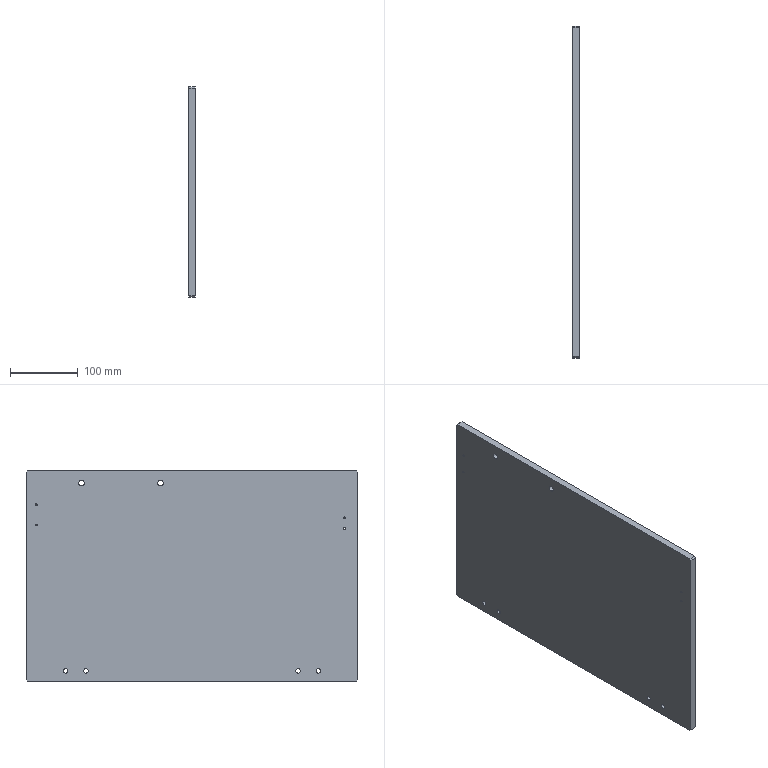Part | STEP file | 227H056119 DOOR R_Default | 1 solid | 30 faces | box 10 x 491 x 311 mm | volume 1524271 mm3 | cylinder 20 | plane 10 | commonest cylinder face diameters 2.5 x8 6.5 x8 8.5 x4